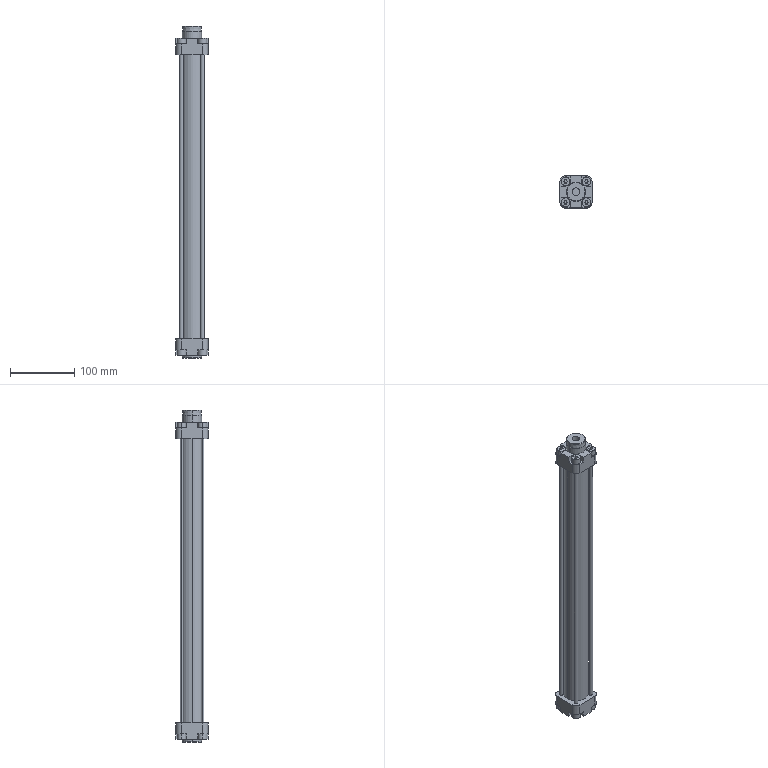Part | STEP file | 1 solid | 306 faces | box 50 x 50 x 517 mm | volume 322395 mm3 | plane 168 | cylinder 86 | cone 36 | torus 16 | commonest cylinder face diameters 4.917 x16 14 x16 6 x12 15.05 x8 17.5 x8 5.9 x4